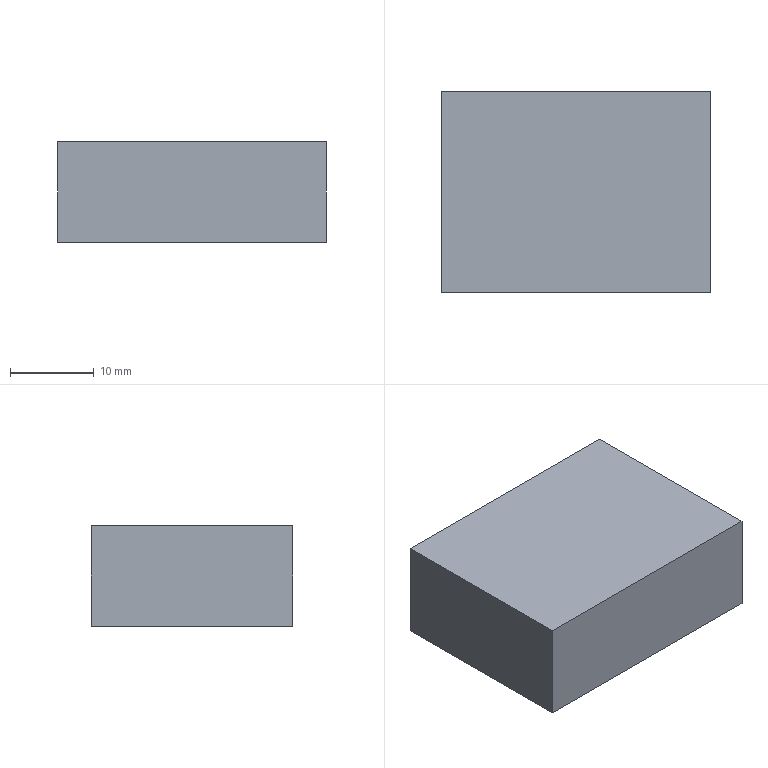Part | SolidWorks | features Extrusion 1 | 1 solid | 6 faces | box 32 x 24 x 12 mm | volume 9216 mm3 | plane 6
STEP:
#1=CARTESIAN_POINT('',(-16.,12.,6.));
#2=VERTEX_POINT('',#1);
#3=CARTESIAN_POINT('',(-16.,-12.,6.));
#4=VERTEX_POINT('',#3);
#5=CARTESIAN_POINT('',(-16.,12.,6.));
#6=DIRECTION('',(0.,-1.,0.));
#7=VECTOR('',#6,1000.);
#8=LINE('',#5,#7);
#9=EDGE_CURVE('',#2,#4,#8,.T.);
#10=ORIENTED_EDGE('',*,*,#9,.F.);
#11=CARTESIAN_POINT('',(-16.,12.,-6.));
#12=VERTEX_POINT('',#11);
#13=CARTESIAN_POINT('',(-16.,12.,-6.));
#14=DIRECTION('',(0.,0.,1.));
#15=VECTOR('',#14,1000.);
#16=LINE('',#13,#15);
#17=EDGE_CURVE('',#12,#2,#16,.T.);
#18=ORIENTED_EDGE('',*,*,#17,.F.);
#19=CARTESIAN_POINT('',(-16.,-12.,-6.));
#20=VERTEX_POINT('',#19);
#21=CARTESIAN_POINT('',(-16.,12.,-6.));
#22=DIRECTION('',(0.,-1.,0.));
#23=VECTOR('',#22,1000.);
#24=LINE('',#21,#23);
#25=EDGE_CURVE('',#12,#20,#24,.T.);
#26=ORIENTED_EDGE('',*,*,#25,.T.);
#27=CARTESIAN_POINT('',(-16.,-12.,-6.));
#28=DIRECTION('',(0.,0.,1.));
#29=VECTOR('',#28,1000.);
#30=LINE('',#27,#29);
#31=EDGE_CURVE('',#20,#4,#30,.T.);
#32=ORIENTED_EDGE('',*,*,#31,.T.);
#33=EDGE_LOOP('',(#10,#18,#26,#32));
#34=FACE_OUTER_BOUND('',#33,.T.);
#35=CARTESIAN_POINT('',(-16.,12.,-6.));
#36=DIRECTION('',(-1.,0.,0.));
#37=DIRECTION('',(0.,0.,1.));
#38=AXIS2_PLACEMENT_3D('',#35,#36,#37);
#39=PLANE('',#38);
#40=ADVANCED_FACE('',(#34),#39,.T.);
#41=CARTESIAN_POINT('',(16.,12.,6.));
#42=VERTEX_POINT('',#41);
#43=CARTESIAN_POINT('',(16.,12.,6.));
#44=DIRECTION('',(-1.,0.,0.));
#45=VECTOR('',#44,1000.);
#46=LINE('',#43,#45);
#47=EDGE_CURVE('',#42,#2,#46,.T.);
#48=ORIENTED_EDGE('',*,*,#47,.F.);
#49=CARTESIAN_POINT('',(16.,12.,-6.));
#50=VERTEX_POINT('',#49);
#51=CARTESIAN_POINT('',(16.,12.,-6.));
#52=DIRECTION('',(0.,0.,1.));
#53=VECTOR('',#52,1000.);
#54=LINE('',#51,#53);
#55=EDGE_CURVE('',#50,#42,#54,.T.);
#56=ORIENTED_EDGE('',*,*,#55,.F.);
#57=CARTESIAN_POINT('',(16.,12.,-6.));
#58=DIRECTION('',(-1.,0.,0.));
#59=VECTOR('',#58,1000.);
#60=LINE('',#57,#59);
#61=EDGE_CURVE('',#50,#12,#60,.T.);
#62=ORIENTED_EDGE('',*,*,#61,.T.);
#63=ORIENTED_EDGE('',*,*,#17,.T.);
#64=EDGE_LOOP('',(#48,#56,#62,#63));
#65=FACE_OUTER_BOUND('',#64,.T.);
#66=CARTESIAN_POINT('',(16.,12.,-6.));
#67=DIRECTION('',(0.,1.,0.));
#68=DIRECTION('',(0.,0.,1.));
#69=AXIS2_PLACEMENT_3D('',#66,#67,#68);
#70=PLANE('',#69);
#71=ADVANCED_FACE('',(#65),#70,.T.);
#72=CARTESIAN_POINT('',(16.,-12.,6.));
#73=VERTEX_POINT('',#72);
#74=CARTESIAN_POINT('',(16.,-12.,6.));
#75=DIRECTION('',(0.,1.,0.));
#76=VECTOR('',#75,1000.);
#77=LINE('',#74,#76);
#78=EDGE_CURVE('',#73,#42,#77,.T.);
#79=ORIENTED_EDGE('',*,*,#78,.F.);
#80=CARTESIAN_POINT('',(16.,-12.,-6.));
#81=VERTEX_POINT('',#80);
#82=CARTESIAN_POINT('',(16.,-12.,-6.));
#83=DIRECTION('',(0.,0.,1.));
#84=VECTOR('',#83,1000.);
#85=LINE('',#82,#84);
#86=EDGE_CURVE('',#81,#73,#85,.T.);
#87=ORIENTED_EDGE('',*,*,#86,.F.);
#88=CARTESIAN_POINT('',(16.,-12.,-6.));
#89=DIRECTION('',(0.,1.,0.));
#90=VECTOR('',#89,1000.);
#91=LINE('',#88,#90);
#92=EDGE_CURVE('',#81,#50,#91,.T.);
#93=ORIENTED_EDGE('',*,*,#92,.T.);
#94=ORIENTED_EDGE('',*,*,#55,.T.);
#95=EDGE_LOOP('',(#79,#87,#93,#94));
#96=FACE_OUTER_BOUND('',#95,.T.);
#97=CARTESIAN_POINT('',(16.,-12.,-6.));
#98=DIRECTION('',(1.,0.,0.));
#99=DIRECTION('',(0.,0.,-1.));
#100=AXIS2_PLACEMENT_3D('',#97,#98,#99);
#101=PLANE('',#100);
#102=ADVANCED_FACE('',(#96),#101,.T.);
#103=CARTESIAN_POINT('',(-16.,-12.,6.));
#104=DIRECTION('',(1.,0.,0.));
#105=VECTOR('',#104,1000.);
#106=LINE('',#103,#105);
#107=EDGE_CURVE('',#4,#73,#106,.T.);
#108=ORIENTED_EDGE('',*,*,#107,.F.);
#109=ORIENTED_EDGE('',*,*,#31,.F.);
#110=CARTESIAN_POINT('',(-16.,-12.,-6.));
#111=DIRECTION('',(1.,0.,0.));
#112=VECTOR('',#111,1000.);
#113=LINE('',#110,#112);
#114=EDGE_CURVE('',#20,#81,#113,.T.);
#115=ORIENTED_EDGE('',*,*,#114,.T.);
#116=ORIENTED_EDGE('',*,*,#86,.T.);
#117=EDGE_LOOP('',(#108,#109,#115,#116));
#118=FACE_OUTER_BOUND('',#117,.T.);
#119=CARTESIAN_POINT('',(-16.,-12.,-6.));
#120=DIRECTION('',(0.,-1.,0.));
#121=DIRECTION('',(0.,0.,-1.));
#122=AXIS2_PLACEMENT_3D('',#119,#120,#121);
#123=PLANE('',#122);
#124=ADVANCED_FACE('',(#118),#123,.T.);
#125=ORIENTED_EDGE('',*,*,#25,.F.);
#126=ORIENTED_EDGE('',*,*,#61,.F.);
#127=ORIENTED_EDGE('',*,*,#92,.F.);
#128=ORIENTED_EDGE('',*,*,#114,.F.);
#129=EDGE_LOOP('',(#125,#126,#127,#128));
#130=FACE_OUTER_BOUND('',#129,.T.);
#131=CARTESIAN_POINT('',(0.,0.,-6.));
#132=DIRECTION('',(0.,0.,1.));
#133=DIRECTION('',(1.,0.,0.));
#134=AXIS2_PLACEMENT_3D('',#131,#132,#133);
#135=PLANE('',#134);
#136=ADVANCED_FACE('',(#130),#135,.F.);
#137=ORIENTED_EDGE('',*,*,#9,.T.);
#138=ORIENTED_EDGE('',*,*,#107,.T.);
#139=ORIENTED_EDGE('',*,*,#78,.T.);
#140=ORIENTED_EDGE('',*,*,#47,.T.);
#141=EDGE_LOOP('',(#137,#138,#139,#140));
#142=FACE_OUTER_BOUND('',#141,.T.);
#143=CARTESIAN_POINT('',(0.,0.,6.));
#144=DIRECTION('',(0.,0.,1.));
#145=DIRECTION('',(1.,0.,0.));
#146=AXIS2_PLACEMENT_3D('',#143,#144,#145);
#147=PLANE('',#146);
#148=ADVANCED_FACE('',(#142),#147,.T.);
#149=CLOSED_SHELL('',(#40,#71,#102,#124,#136,#148));
#150=MANIFOLD_SOLID_BREP('',#149);
#151=CARTESIAN_POINT('',(0.,0.,0.));
#152=DIRECTION('',(0.,0.,1.));
#153=DIRECTION('',(1.,0.,0.));
#154=AXIS2_PLACEMENT_3D('',#151,#152,#153);
#155=(LENGTH_UNIT()NAMED_UNIT(*)SI_UNIT(.MILLI.,.METRE.));
#156=UNCERTAINTY_MEASURE_WITH_UNIT(LENGTH_MEASURE(0.00001),#155,'','');
#157=(NAMED_UNIT(*)PLANE_ANGLE_UNIT()SI_UNIT($,.RADIAN.));
#158=(NAMED_UNIT(*)SI_UNIT($,.STERADIAN.)SOLID_ANGLE_UNIT());
#159=(GEOMETRIC_REPRESENTATION_CONTEXT(3)GLOBAL_UNCERTAINTY_ASSIGNED_CONTEXT((#156))GLOBAL_UNIT_ASSIGNED_CONTEXT((#155,#157,#158))REPRESENTATION_CONTEXT('',''));
#160=ADVANCED_BREP_SHAPE_REPRESENTATION('',(#150,#154),#159);